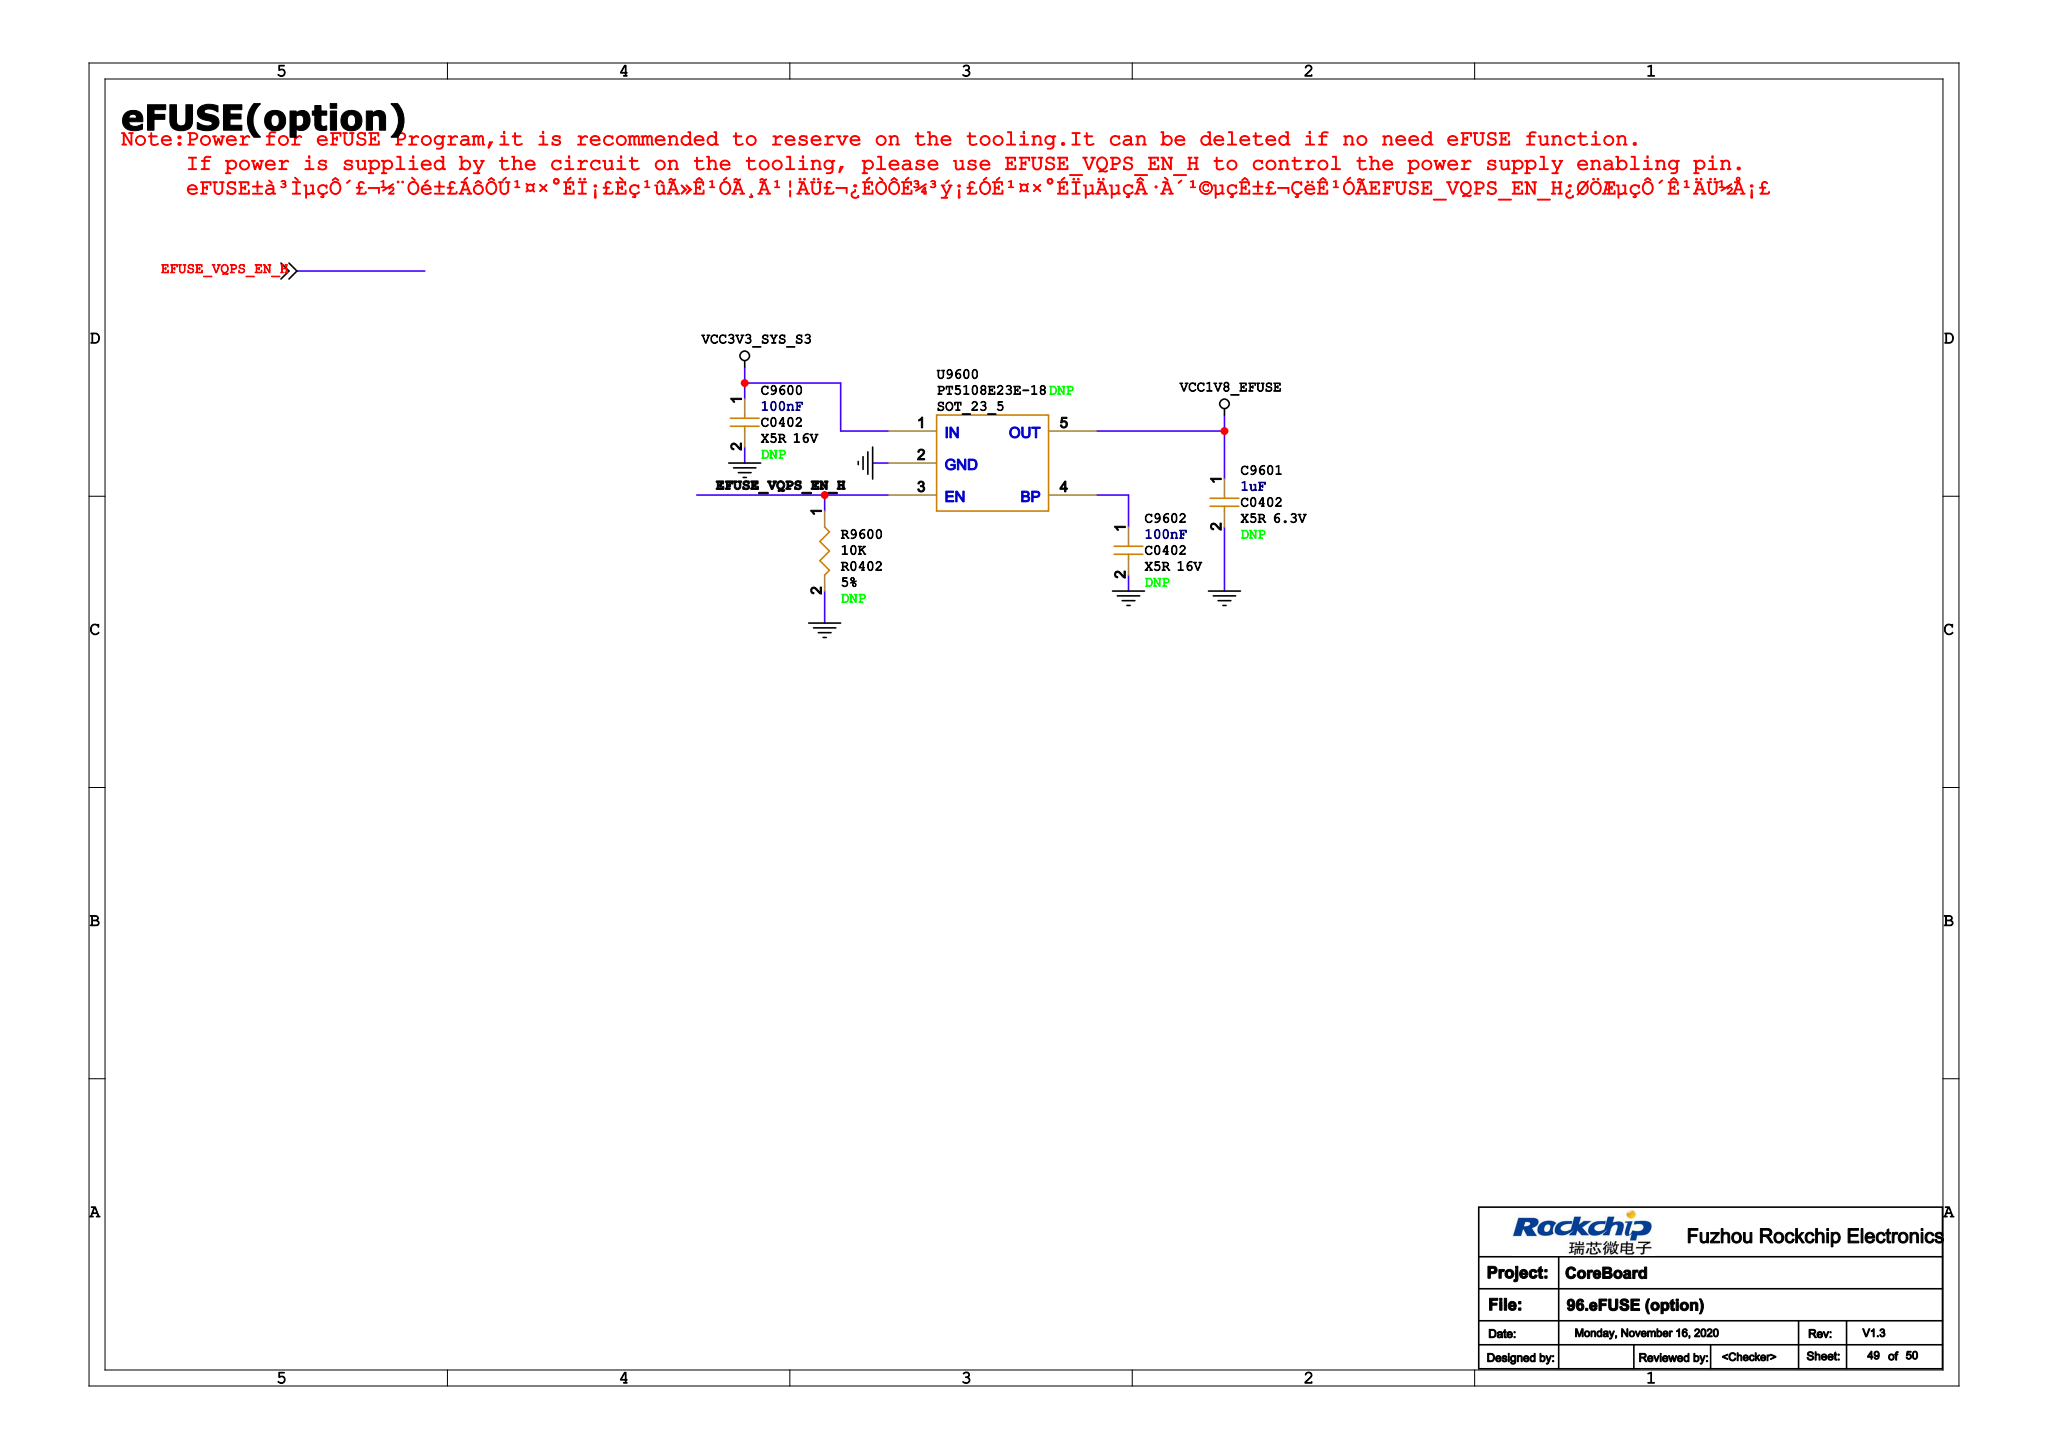Circuit board | Cadence Allegro | 749 parts | 717 nets | one sheet of the schematic
Parts on this sheet (reference | value | footprint):
C9600 | 100nF | C0402
C9601 | 1uF | C0402
C9602 | 100nF | C0402
R9600 | 10K | R0402
U9600 | PT5108E23E-18 | SOT_23_5
Nets of these parts (net: part-pin ...):
GND: C9600-2 C9601-2 C9602-2 R9600-2 U9600-2
VCC3V3_SYS_S3: C9600-1 U9600-1
VCC1V8_EFUSE: C9601-1 U9600-5
EFUSE_VQPS_EN_H: R9600-1 U9600-3
N77675235: C9602-1 U9600-4